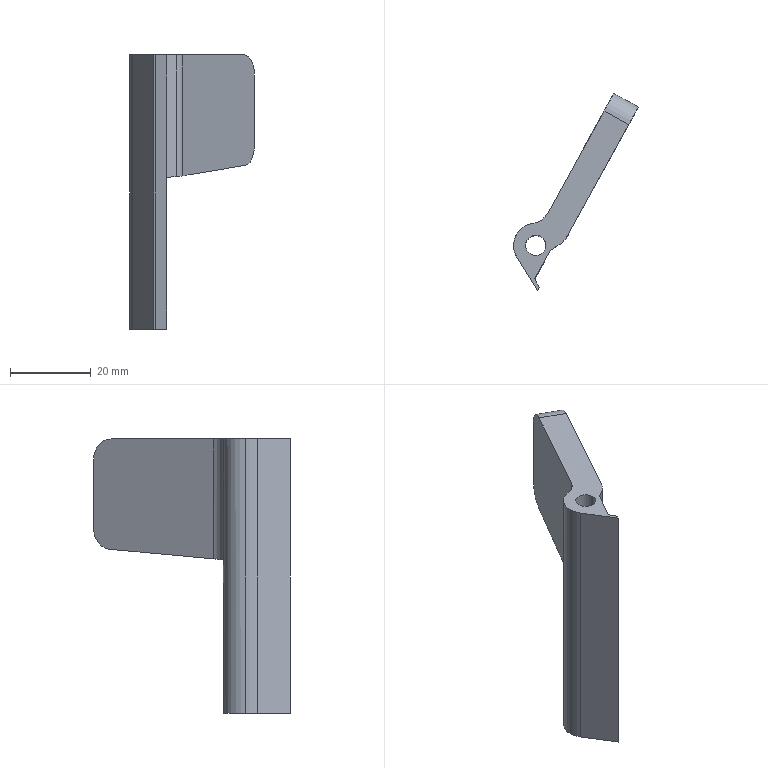Part | SolidWorks | features BaseBody 1 | 1 solid | 21 faces | box 30.974 x 48.805 x 68 mm | volume 12607 mm3 | plane 13 | cylinder 8 | commonest cylinder face diameters 10 x4 5 x2 11 x2
STEP:
#1=CARTESIAN_POINT('',(-2.751,-1.776,34.));
#2=VERTEX_POINT('',#1);
#3=CARTESIAN_POINT('',(-1.932,-4.664,34.));
#4=VERTEX_POINT('',#3);
#5=CARTESIAN_POINT('',(2.749,-1.776,34.));
#6=DIRECTION('',(0.,0.,1.));
#7=DIRECTION('',(-1.,0.,0.));
#8=AXIS2_PLACEMENT_3D('',#5,#6,#7);
#9=CIRCLE('',#8,5.5);
#10=EDGE_CURVE('',#2,#4,#9,.T.);
#11=ORIENTED_EDGE('',*,*,#10,.F.);
#12=CARTESIAN_POINT('',(-2.751,-1.776,-34.));
#13=VERTEX_POINT('',#12);
#14=CARTESIAN_POINT('',(-2.751,-1.776,34.));
#15=DIRECTION('',(0.,0.,-1.));
#16=VECTOR('',#15,1000.);
#17=LINE('',#14,#16);
#18=EDGE_CURVE('',#2,#13,#17,.T.);
#19=ORIENTED_EDGE('',*,*,#18,.T.);
#20=CARTESIAN_POINT('',(-1.932,-4.664,-34.));
#21=VERTEX_POINT('',#20);
#22=CARTESIAN_POINT('',(2.749,-1.776,-34.));
#23=DIRECTION('',(0.,0.,1.));
#24=DIRECTION('',(-1.,0.,0.));
#25=AXIS2_PLACEMENT_3D('',#22,#23,#24);
#26=CIRCLE('',#25,5.5);
#27=EDGE_CURVE('',#13,#21,#26,.T.);
#28=ORIENTED_EDGE('',*,*,#27,.T.);
#29=CARTESIAN_POINT('',(-1.932,-4.664,34.));
#30=DIRECTION('',(0.,0.,1.));
#31=VECTOR('',#30,1000.);
#32=LINE('',#29,#31);
#33=EDGE_CURVE('',#21,#4,#32,.T.);
#34=ORIENTED_EDGE('',*,*,#33,.T.);
#35=EDGE_LOOP('',(#11,#19,#28,#34));
#36=FACE_OUTER_BOUND('',#35,.T.);
#37=CARTESIAN_POINT('',(2.749,-1.776,34.));
#38=DIRECTION('',(0.,0.,-1.));
#39=DIRECTION('',(-1.,0.,0.));
#40=AXIS2_PLACEMENT_3D('',#37,#38,#39);
#41=CYLINDRICAL_SURFACE('',#40,5.5);
#42=ADVANCED_FACE('',(#36),#41,.T.);
#43=CARTESIAN_POINT('',(0.2488,-1.776,-34.));
#44=VERTEX_POINT('',#43);
#45=CARTESIAN_POINT('',(5.249,-1.776,-34.));
#46=VERTEX_POINT('',#45);
#47=CARTESIAN_POINT('',(2.749,-1.776,-34.));
#48=DIRECTION('',(0.,0.,1.));
#49=DIRECTION('',(1.,0.,0.));
#50=AXIS2_PLACEMENT_3D('',#47,#48,#49);
#51=CIRCLE('',#50,2.5);
#52=EDGE_CURVE('',#44,#46,#51,.T.);
#53=ORIENTED_EDGE('',*,*,#52,.F.);
#54=CARTESIAN_POINT('',(0.2488,-1.776,34.));
#55=VERTEX_POINT('',#54);
#56=CARTESIAN_POINT('',(0.2488,-1.776,-34.));
#57=DIRECTION('',(0.,0.,1.));
#58=VECTOR('',#57,1000.);
#59=LINE('',#56,#58);
#60=EDGE_CURVE('',#44,#55,#59,.T.);
#61=ORIENTED_EDGE('',*,*,#60,.T.);
#62=CARTESIAN_POINT('',(5.249,-1.776,34.));
#63=VERTEX_POINT('',#62);
#64=CARTESIAN_POINT('',(2.749,-1.776,34.));
#65=DIRECTION('',(0.,0.,-1.));
#66=DIRECTION('',(1.,0.,0.));
#67=AXIS2_PLACEMENT_3D('',#64,#65,#66);
#68=CIRCLE('',#67,2.5);
#69=EDGE_CURVE('',#63,#55,#68,.T.);
#70=ORIENTED_EDGE('',*,*,#69,.F.);
#71=CARTESIAN_POINT('',(5.249,-1.776,-34.));
#72=DIRECTION('',(0.,0.,1.));
#73=VECTOR('',#72,1000.);
#74=LINE('',#71,#73);
#75=EDGE_CURVE('',#46,#63,#74,.T.);
#76=ORIENTED_EDGE('',*,*,#75,.F.);
#77=EDGE_LOOP('',(#53,#61,#70,#76));
#78=FACE_OUTER_BOUND('',#77,.T.);
#79=CARTESIAN_POINT('',(2.749,-1.776,-34.));
#80=DIRECTION('',(0.,0.,1.));
#81=DIRECTION('',(1.,0.,0.));
#82=AXIS2_PLACEMENT_3D('',#79,#80,#81);
#83=CYLINDRICAL_SURFACE('',#82,2.5);
#84=ADVANCED_FACE('',(#78),#83,.F.);
#85=CARTESIAN_POINT('',(26.006,28.527,6.627));
#86=VERTEX_POINT('',#85);
#87=CARTESIAN_POINT('',(10.493,0.3506,4.019));
#88=VERTEX_POINT('',#87);
#89=CARTESIAN_POINT('',(26.006,28.527,6.627));
#90=DIRECTION('',(-0.4807,-0.8731,-0.08082));
#91=VECTOR('',#90,1000.);
#92=LINE('',#89,#91);
#93=EDGE_CURVE('',#86,#88,#92,.T.);
#94=ORIENTED_EDGE('',*,*,#93,.F.);
#95=CARTESIAN_POINT('',(28.223,32.553,11.611));
#96=VERTEX_POINT('',#95);
#97=CARTESIAN_POINT('',(25.811,28.173,11.611));
#98=DIRECTION('',(-0.876,0.4823,0.));
#99=DIRECTION('',(0.4823,0.876,0.));
#100=AXIS2_PLACEMENT_3D('',#97,#98,#99);
#101=CIRCLE('',#100,5.);
#102=EDGE_CURVE('',#96,#86,#101,.T.);
#103=ORIENTED_EDGE('',*,*,#102,.F.);
#104=CARTESIAN_POINT('',(28.223,32.553,29.));
#105=VERTEX_POINT('',#104);
#106=CARTESIAN_POINT('',(28.223,32.553,34.));
#107=DIRECTION('',(0.,0.,-1.));
#108=VECTOR('',#107,1000.);
#109=LINE('',#106,#108);
#110=EDGE_CURVE('',#105,#96,#109,.T.);
#111=ORIENTED_EDGE('',*,*,#110,.F.);
#112=CARTESIAN_POINT('',(25.811,28.173,34.));
#113=VERTEX_POINT('',#112);
#114=CARTESIAN_POINT('',(25.811,28.173,29.));
#115=DIRECTION('',(-0.876,0.4823,0.));
#116=DIRECTION('',(0.4823,0.876,0.));
#117=AXIS2_PLACEMENT_3D('',#114,#115,#116);
#118=CIRCLE('',#117,5.);
#119=EDGE_CURVE('',#113,#105,#118,.T.);
#120=ORIENTED_EDGE('',*,*,#119,.F.);
#121=CARTESIAN_POINT('',(10.493,0.3506,34.));
#122=VERTEX_POINT('',#121);
#123=CARTESIAN_POINT('',(28.223,32.553,34.));
#124=DIRECTION('',(0.4823,0.876,0.));
#125=VECTOR('',#124,1000.);
#126=LINE('',#123,#125);
#127=EDGE_CURVE('',#122,#113,#126,.T.);
#128=ORIENTED_EDGE('',*,*,#127,.F.);
#129=CARTESIAN_POINT('',(10.493,0.3506,34.));
#130=DIRECTION('',(0.,0.,1.));
#131=VECTOR('',#130,1000.);
#132=LINE('',#129,#131);
#133=EDGE_CURVE('',#88,#122,#132,.T.);
#134=ORIENTED_EDGE('',*,*,#133,.F.);
#135=EDGE_LOOP('',(#94,#103,#111,#120,#128,#134));
#136=FACE_OUTER_BOUND('',#135,.T.);
#137=CARTESIAN_POINT('',(28.223,32.553,34.));
#138=DIRECTION('',(-0.876,0.4823,0.));
#139=DIRECTION('',(-0.4823,-0.876,0.));
#140=AXIS2_PLACEMENT_3D('',#137,#138,#139);
#141=PLANE('',#140);
#142=ADVANCED_FACE('',(#136),#141,.F.);
#143=CARTESIAN_POINT('',(8.818,-1.443,34.));
#144=VERTEX_POINT('',#143);
#145=CARTESIAN_POINT('',(8.818,-1.443,3.827));
#146=VERTEX_POINT('',#145);
#147=CARTESIAN_POINT('',(8.818,-1.443,-47.577));
#148=DIRECTION('',(0.,0.,-1.));
#149=VECTOR('',#148,1000.);
#150=LINE('',#147,#149);
#151=EDGE_CURVE('',#144,#146,#150,.T.);
#152=ORIENTED_EDGE('',*,*,#151,.T.);
#153=CARTESIAN_POINT('',(8.818,-1.443,3.827));
#154=CARTESIAN_POINT('',(9.52,-0.9916,3.886));
#155=CARTESIAN_POINT('',(10.09,-0.3811,3.952));
#156=CARTESIAN_POINT('',(10.493,0.3506,4.019));
#157=(BOUNDED_CURVE()B_SPLINE_CURVE(3,(#153,#154,#155,#156),.UNSPECIFIED.,.F.,.F.)B_SPLINE_CURVE_WITH_KNOTS((4,4),(4.216,4.712),.UNSPECIFIED.)CURVE()GEOMETRIC_REPRESENTATION_ITEM()RATIONAL_B_SPLINE_CURVE((1.,0.9796,0.9796,1.))REPRESENTATION_ITEM(''));
#158=EDGE_CURVE('',#146,#88,#157,.T.);
#159=ORIENTED_EDGE('',*,*,#158,.T.);
#160=ORIENTED_EDGE('',*,*,#133,.T.);
#161=CARTESIAN_POINT('',(6.113,2.762,34.));
#162=DIRECTION('',(0.,0.,-1.));
#163=DIRECTION('',(1.,0.,0.));
#164=AXIS2_PLACEMENT_3D('',#161,#162,#163);
#165=CIRCLE('',#164,5.);
#166=EDGE_CURVE('',#122,#144,#165,.T.);
#167=ORIENTED_EDGE('',*,*,#166,.T.);
#168=EDGE_LOOP('',(#152,#159,#160,#167));
#169=FACE_OUTER_BOUND('',#168,.T.);
#170=CARTESIAN_POINT('',(6.113,2.762,-47.577));
#171=DIRECTION('',(0.,0.,1.));
#172=DIRECTION('',(1.,0.,0.));
#173=AXIS2_PLACEMENT_3D('',#170,#171,#172);
#174=CYLINDRICAL_SURFACE('',#173,5.);
#175=ADVANCED_FACE('',(#169),#174,.T.);
#176=CARTESIAN_POINT('',(4.245,3.517,4.));
#177=VERTEX_POINT('',#176);
#178=CARTESIAN_POINT('',(2.018,3.675,3.924));
#179=VERTEX_POINT('',#178);
#180=CARTESIAN_POINT('',(4.245,3.517,4.));
#181=CARTESIAN_POINT('',(3.519,3.722,3.986));
#182=CARTESIAN_POINT('',(2.766,3.776,3.961));
#183=CARTESIAN_POINT('',(2.018,3.675,3.924));
#184=(BOUNDED_CURVE()B_SPLINE_CURVE(3,(#180,#181,#182,#183),.UNSPECIFIED.,.F.,.F.)B_SPLINE_CURVE_WITH_KNOTS((4,4),(3.369,3.778),.UNSPECIFIED.)CURVE()GEOMETRIC_REPRESENTATION_ITEM()RATIONAL_B_SPLINE_CURVE((1.,0.9861,0.9861,1.))REPRESENTATION_ITEM(''));
#185=EDGE_CURVE('',#177,#179,#184,.T.);
#186=ORIENTED_EDGE('',*,*,#185,.T.);
#187=CARTESIAN_POINT('',(5.734,6.22,4.25));
#188=VERTEX_POINT('',#187);
#189=CARTESIAN_POINT('',(2.018,3.675,3.924));
#190=CARTESIAN_POINT('',(3.62,3.89,4.002));
#191=CARTESIAN_POINT('',(4.954,4.803,4.119));
#192=CARTESIAN_POINT('',(5.734,6.22,4.25));
#193=(BOUNDED_CURVE()B_SPLINE_CURVE(3,(#189,#190,#191,#192),.UNSPECIFIED.,.F.,.F.)B_SPLINE_CURVE_WITH_KNOTS((4,4),(0.6366,1.571),.UNSPECIFIED.)CURVE()GEOMETRIC_REPRESENTATION_ITEM()RATIONAL_B_SPLINE_CURVE((1.,0.9286,0.9286,1.))REPRESENTATION_ITEM(''));
#194=EDGE_CURVE('',#179,#188,#193,.T.);
#195=ORIENTED_EDGE('',*,*,#194,.T.);
#196=CARTESIAN_POINT('',(19.874,31.903,6.627));
#197=VERTEX_POINT('',#196);
#198=CARTESIAN_POINT('',(5.734,6.22,4.25));
#199=DIRECTION('',(0.4807,0.8731,0.08082));
#200=VECTOR('',#199,1000.);
#201=LINE('',#198,#200);
#202=EDGE_CURVE('',#188,#197,#201,.T.);
#203=ORIENTED_EDGE('',*,*,#202,.T.);
#204=CARTESIAN_POINT('',(19.874,31.903,6.627));
#205=DIRECTION('',(0.876,-0.4823,0.));
#206=VECTOR('',#205,1000.);
#207=LINE('',#204,#206);
#208=EDGE_CURVE('',#197,#86,#207,.T.);
#209=ORIENTED_EDGE('',*,*,#208,.T.);
#210=ORIENTED_EDGE('',*,*,#93,.T.);
#211=ORIENTED_EDGE('',*,*,#158,.F.);
#212=CARTESIAN_POINT('',(6.348,-3.031,3.617));
#213=VERTEX_POINT('',#212);
#214=CARTESIAN_POINT('',(8.818,-1.443,3.827));
#215=DIRECTION('',(-0.839,-0.5395,-0.07113));
#216=VECTOR('',#215,1000.);
#217=LINE('',#214,#216);
#218=EDGE_CURVE('',#146,#213,#217,.T.);
#219=ORIENTED_EDGE('',*,*,#218,.T.);
#220=CARTESIAN_POINT('',(6.421,2.319,4.));
#221=VERTEX_POINT('',#220);
#222=CARTESIAN_POINT('',(6.348,-3.031,3.617));
#223=DIRECTION('',(0.01357,0.9974,0.07137));
#224=VECTOR('',#223,1000.);
#225=LINE('',#222,#224);
#226=EDGE_CURVE('',#213,#221,#225,.T.);
#227=ORIENTED_EDGE('',*,*,#226,.T.);
#228=CARTESIAN_POINT('',(6.421,2.319,4.));
#229=DIRECTION('',(-0.876,0.4823,0.));
#230=VECTOR('',#229,1000.);
#231=LINE('',#228,#230);
#232=EDGE_CURVE('',#221,#177,#231,.T.);
#233=ORIENTED_EDGE('',*,*,#232,.T.);
#234=EDGE_LOOP('',(#186,#195,#203,#209,#210,#211,#219,#227,#233));
#235=FACE_OUTER_BOUND('',#234,.T.);
#236=CARTESIAN_POINT('',(21.765,-6.13,4.));
#237=DIRECTION('',(0.03898,0.07079,-0.9967));
#238=DIRECTION('',(0.,0.9975,0.07085));
#239=AXIS2_PLACEMENT_3D('',#236,#237,#238);
#240=PLANE('',#239);
#241=ADVANCED_FACE('',(#235),#240,.T.);
#242=ORIENTED_EDGE('',*,*,#102,.T.);
#243=ORIENTED_EDGE('',*,*,#208,.F.);
#244=CARTESIAN_POINT('',(22.091,35.929,11.611));
#245=VERTEX_POINT('',#244);
#246=CARTESIAN_POINT('',(19.679,31.549,11.611));
#247=DIRECTION('',(0.876,-0.4823,0.));
#248=DIRECTION('',(0.4823,0.876,0.));
#249=AXIS2_PLACEMENT_3D('',#246,#247,#248);
#250=CIRCLE('',#249,5.);
#251=EDGE_CURVE('',#197,#245,#250,.T.);
#252=ORIENTED_EDGE('',*,*,#251,.T.);
#253=CARTESIAN_POINT('',(28.223,32.553,11.611));
#254=DIRECTION('',(0.876,-0.4823,0.));
#255=VECTOR('',#254,1000.);
#256=LINE('',#253,#255);
#257=EDGE_CURVE('',#245,#96,#256,.T.);
#258=ORIENTED_EDGE('',*,*,#257,.T.);
#259=EDGE_LOOP('',(#242,#243,#252,#258));
#260=FACE_OUTER_BOUND('',#259,.T.);
#261=CARTESIAN_POINT('',(25.811,28.173,11.611));
#262=DIRECTION('',(0.876,-0.4823,0.));
#263=DIRECTION('',(0.4823,0.876,0.));
#264=AXIS2_PLACEMENT_3D('',#261,#262,#263);
#265=CYLINDRICAL_SURFACE('',#264,5.);
#266=ADVANCED_FACE('',(#260),#265,.T.);
#267=CARTESIAN_POINT('',(22.091,35.929,29.));
#268=VERTEX_POINT('',#267);
#269=CARTESIAN_POINT('',(22.091,35.929,34.));
#270=DIRECTION('',(0.,0.,-1.));
#271=VECTOR('',#270,1000.);
#272=LINE('',#269,#271);
#273=EDGE_CURVE('',#268,#245,#272,.T.);
#274=ORIENTED_EDGE('',*,*,#273,.F.);
#275=CARTESIAN_POINT('',(28.223,32.553,29.));
#276=DIRECTION('',(-0.876,0.4823,0.));
#277=VECTOR('',#276,1000.);
#278=LINE('',#275,#277);
#279=EDGE_CURVE('',#105,#268,#278,.T.);
#280=ORIENTED_EDGE('',*,*,#279,.F.);
#281=ORIENTED_EDGE('',*,*,#110,.T.);
#282=ORIENTED_EDGE('',*,*,#257,.F.);
#283=EDGE_LOOP('',(#274,#280,#281,#282));
#284=FACE_OUTER_BOUND('',#283,.T.);
#285=CARTESIAN_POINT('',(28.223,32.553,34.));
#286=DIRECTION('',(-0.4823,-0.876,0.));
#287=DIRECTION('',(0.876,-0.4823,0.));
#288=AXIS2_PLACEMENT_3D('',#285,#286,#287);
#289=PLANE('',#288);
#290=ADVANCED_FACE('',(#284),#289,.F.);
#291=ORIENTED_EDGE('',*,*,#119,.T.);
#292=ORIENTED_EDGE('',*,*,#279,.T.);
#293=CARTESIAN_POINT('',(19.679,31.549,34.));
#294=VERTEX_POINT('',#293);
#295=CARTESIAN_POINT('',(19.679,31.549,29.));
#296=DIRECTION('',(0.876,-0.4823,0.));
#297=DIRECTION('',(0.4823,0.876,0.));
#298=AXIS2_PLACEMENT_3D('',#295,#296,#297);
#299=CIRCLE('',#298,5.);
#300=EDGE_CURVE('',#268,#294,#299,.T.);
#301=ORIENTED_EDGE('',*,*,#300,.T.);
#302=CARTESIAN_POINT('',(20.767,30.95,34.));
#303=DIRECTION('',(0.876,-0.4823,0.));
#304=VECTOR('',#303,1000.);
#305=LINE('',#302,#304);
#306=EDGE_CURVE('',#294,#113,#305,.T.);
#307=ORIENTED_EDGE('',*,*,#306,.T.);
#308=EDGE_LOOP('',(#291,#292,#301,#307));
#309=FACE_OUTER_BOUND('',#308,.T.);
#310=CARTESIAN_POINT('',(20.767,30.95,29.));
#311=DIRECTION('',(0.876,-0.4823,0.));
#312=DIRECTION('',(0.4823,0.876,0.));
#313=AXIS2_PLACEMENT_3D('',#310,#311,#312);
#314=CYLINDRICAL_SURFACE('',#313,5.);
#315=ADVANCED_FACE('',(#309),#314,.T.);
#316=CARTESIAN_POINT('',(3.211,-12.876,34.));
#317=VERTEX_POINT('',#316);
#318=CARTESIAN_POINT('',(-1.932,-4.664,34.));
#319=DIRECTION('',(0.5308,-0.8475,0.));
#320=VECTOR('',#319,1000.);
#321=LINE('',#318,#320);
#322=EDGE_CURVE('',#4,#317,#321,.T.);
#323=ORIENTED_EDGE('',*,*,#322,.T.);
#324=CARTESIAN_POINT('',(3.612,-12.147,34.));
#325=VERTEX_POINT('',#324);
#326=CARTESIAN_POINT('',(28.223,32.553,34.));
#327=DIRECTION('',(0.4823,0.876,0.));
#328=VECTOR('',#327,1000.);
#329=LINE('',#326,#328);
#330=EDGE_CURVE('',#317,#325,#329,.T.);
#331=ORIENTED_EDGE('',*,*,#330,.T.);
#332=CARTESIAN_POINT('',(2.489,-10.039,34.));
#333=VERTEX_POINT('',#332);
#334=CARTESIAN_POINT('',(3.612,-12.147,34.));
#335=DIRECTION('',(-0.4703,0.8825,0.));
#336=VECTOR('',#335,1000.);
#337=LINE('',#334,#336);
#338=EDGE_CURVE('',#325,#333,#337,.T.);
#339=ORIENTED_EDGE('',*,*,#338,.T.);
#340=CARTESIAN_POINT('',(6.348,-3.031,34.));
#341=VERTEX_POINT('',#340);
#342=CARTESIAN_POINT('',(2.489,-10.039,34.));
#343=DIRECTION('',(0.4823,0.876,0.));
#344=VECTOR('',#343,1000.);
#345=LINE('',#342,#344);
#346=EDGE_CURVE('',#333,#341,#345,.T.);
#347=ORIENTED_EDGE('',*,*,#346,.T.);
#348=CARTESIAN_POINT('',(6.348,-3.031,34.));
#349=DIRECTION('',(0.8411,0.5409,0.));
#350=VECTOR('',#349,1000.);
#351=LINE('',#348,#350);
#352=EDGE_CURVE('',#341,#144,#351,.T.);
#353=ORIENTED_EDGE('',*,*,#352,.T.);
#354=ORIENTED_EDGE('',*,*,#166,.F.);
#355=ORIENTED_EDGE('',*,*,#127,.T.);
#356=ORIENTED_EDGE('',*,*,#306,.F.);
#357=CARTESIAN_POINT('',(5.734,6.22,34.));
#358=VERTEX_POINT('',#357);
#359=CARTESIAN_POINT('',(19.679,31.549,34.));
#360=DIRECTION('',(-0.4823,-0.876,0.));
#361=VECTOR('',#360,1000.);
#362=LINE('',#359,#361);
#363=EDGE_CURVE('',#294,#358,#362,.T.);
#364=ORIENTED_EDGE('',*,*,#363,.T.);
#365=CARTESIAN_POINT('',(2.018,3.675,34.));
#366=VERTEX_POINT('',#365);
#367=CARTESIAN_POINT('',(1.354,8.631,34.));
#368=DIRECTION('',(0.,0.,-1.));
#369=DIRECTION('',(-1.,0.,0.));
#370=AXIS2_PLACEMENT_3D('',#367,#368,#369);
#371=CIRCLE('',#370,5.);
#372=EDGE_CURVE('',#358,#366,#371,.T.);
#373=ORIENTED_EDGE('',*,*,#372,.T.);
#374=CARTESIAN_POINT('',(2.749,-1.776,34.));
#375=DIRECTION('',(0.,0.,1.));
#376=DIRECTION('',(-1.,0.,0.));
#377=AXIS2_PLACEMENT_3D('',#374,#375,#376);
#378=CIRCLE('',#377,5.5);
#379=EDGE_CURVE('',#366,#2,#378,.T.);
#380=ORIENTED_EDGE('',*,*,#379,.T.);
#381=ORIENTED_EDGE('',*,*,#10,.T.);
#382=EDGE_LOOP('',(#323,#331,#339,#347,#353,#354,#355,#356,#364,#373,#380,#381));
#383=FACE_OUTER_BOUND('',#382,.T.);
#384=ORIENTED_EDGE('',*,*,#69,.T.);
#385=CARTESIAN_POINT('',(2.749,-1.776,34.));
#386=DIRECTION('',(0.,0.,-1.));
#387=DIRECTION('',(1.,0.,0.));
#388=AXIS2_PLACEMENT_3D('',#385,#386,#387);
#389=CIRCLE('',#388,2.5);
#390=EDGE_CURVE('',#55,#63,#389,.T.);
#391=ORIENTED_EDGE('',*,*,#390,.T.);
#392=EDGE_LOOP('',(#384,#391));
#393=FACE_BOUND('',#392,.T.);
#394=CARTESIAN_POINT('',(2.749,-1.776,34.));
#395=DIRECTION('',(0.,0.,1.));
#396=DIRECTION('',(1.,0.,0.));
#397=AXIS2_PLACEMENT_3D('',#394,#395,#396);
#398=PLANE('',#397);
#399=ADVANCED_FACE('',(#383,#393),#398,.T.);
#400=ORIENTED_EDGE('',*,*,#352,.F.);
#401=CARTESIAN_POINT('',(6.348,-3.031,-47.577));
#402=DIRECTION('',(0.,0.,1.));
#403=VECTOR('',#402,1000.);
#404=LINE('',#401,#403);
#405=EDGE_CURVE('',#213,#341,#404,.T.);
#406=ORIENTED_EDGE('',*,*,#405,.F.);
#407=ORIENTED_EDGE('',*,*,#218,.F.);
#408=ORIENTED_EDGE('',*,*,#151,.F.);
#409=EDGE_LOOP('',(#400,#406,#407,#408));
#410=FACE_OUTER_BOUND('',#409,.T.);
#411=CARTESIAN_POINT('',(6.348,-3.031,-47.577));
#412=DIRECTION('',(-0.5409,0.8411,0.));
#413=DIRECTION('',(-0.8411,-0.5409,0.));
#414=AXIS2_PLACEMENT_3D('',#411,#412,#413);
#415=PLANE('',#414);
#416=ADVANCED_FACE('',(#410),#415,.F.);
#417=ORIENTED_EDGE('',*,*,#194,.F.);
#418=CARTESIAN_POINT('',(2.018,3.675,34.));
#419=DIRECTION('',(0.,0.,-1.));
#420=VECTOR('',#419,1000.);
#421=LINE('',#418,#420);
#422=EDGE_CURVE('',#366,#179,#421,.T.);
#423=ORIENTED_EDGE('',*,*,#422,.F.);
#424=ORIENTED_EDGE('',*,*,#372,.F.);
#425=CARTESIAN_POINT('',(5.734,6.22,34.));
#426=DIRECTION('',(0.,0.,1.));
#427=VECTOR('',#426,1000.);
#428=LINE('',#425,#427);
#429=EDGE_CURVE('',#188,#358,#428,.T.);
#430=ORIENTED_EDGE('',*,*,#429,.F.);
#431=EDGE_LOOP('',(#417,#423,#424,#430));
#432=FACE_OUTER_BOUND('',#431,.T.);
#433=CARTESIAN_POINT('',(1.354,8.631,34.));
#434=DIRECTION('',(0.,0.,-1.));
#435=DIRECTION('',(-1.,0.,0.));
#436=AXIS2_PLACEMENT_3D('',#433,#434,#435);
#437=CYLINDRICAL_SURFACE('',#436,5.);
#438=ADVANCED_FACE('',(#432),#437,.F.);
#439=ORIENTED_EDGE('',*,*,#18,.F.);
#440=ORIENTED_EDGE('',*,*,#379,.F.);
#441=ORIENTED_EDGE('',*,*,#422,.T.);
#442=ORIENTED_EDGE('',*,*,#185,.F.);
#443=CARTESIAN_POINT('',(4.245,3.517,-34.));
#444=VERTEX_POINT('',#443);
#445=CARTESIAN_POINT('',(4.245,3.517,34.));
#446=DIRECTION('',(0.,0.,-1.));
#447=VECTOR('',#446,1000.);
#448=LINE('',#445,#447);
#449=EDGE_CURVE('',#177,#444,#448,.T.);
#450=ORIENTED_EDGE('',*,*,#449,.T.);
#451=CARTESIAN_POINT('',(2.749,-1.776,-34.));
#452=DIRECTION('',(0.,0.,1.));
#453=DIRECTION('',(-1.,0.,0.));
#454=AXIS2_PLACEMENT_3D('',#451,#452,#453);
#455=CIRCLE('',#454,5.5);
#456=EDGE_CURVE('',#444,#13,#455,.T.);
#457=ORIENTED_EDGE('',*,*,#456,.T.);
#458=EDGE_LOOP('',(#439,#440,#441,#442,#450,#457));
#459=FACE_OUTER_BOUND('',#458,.T.);
#460=CARTESIAN_POINT('',(2.749,-1.776,34.));
#461=DIRECTION('',(0.,0.,-1.));
#462=DIRECTION('',(-1.,0.,0.));
#463=AXIS2_PLACEMENT_3D('',#460,#461,#462);
#464=CYLINDRICAL_SURFACE('',#463,5.5);
#465=ADVANCED_FACE('',(#459),#464,.T.);
#466=CARTESIAN_POINT('',(6.421,2.319,-34.));
#467=VERTEX_POINT('',#466);
#468=CARTESIAN_POINT('',(6.421,2.319,4.));
#469=DIRECTION('',(0.,0.,-1.));
#470=VECTOR('',#469,1000.);
#471=LINE('',#468,#470);
#472=EDGE_CURVE('',#221,#467,#471,.T.);
#473=ORIENTED_EDGE('',*,*,#472,.T.);
#474=CARTESIAN_POINT('',(21.765,-6.13,-34.));
#475=DIRECTION('',(-0.876,0.4823,0.));
#476=VECTOR('',#475,1000.);
#477=LINE('',#474,#476);
#478=EDGE_CURVE('',#467,#444,#477,.T.);
#479=ORIENTED_EDGE('',*,*,#478,.T.);
#480=ORIENTED_EDGE('',*,*,#449,.F.);
#481=ORIENTED_EDGE('',*,*,#232,.F.);
#482=EDGE_LOOP('',(#473,#479,#480,#481));
#483=FACE_OUTER_BOUND('',#482,.T.);
#484=CARTESIAN_POINT('',(21.765,-6.13,4.));
#485=DIRECTION('',(0.4823,0.876,0.));
#486=DIRECTION('',(-0.876,0.4823,0.));
#487=AXIS2_PLACEMENT_3D('',#484,#485,#486);
#488=PLANE('',#487);
#489=ADVANCED_FACE('',(#483),#488,.T.);
#490=CARTESIAN_POINT('',(6.348,-3.031,-34.));
#491=VERTEX_POINT('',#490);
#492=CARTESIAN_POINT('',(6.348,-3.031,-34.));
#493=DIRECTION('',(-0.01361,-0.9999,0.));
#494=VECTOR('',#493,1000.);
#495=LINE('',#492,#494);
#496=EDGE_CURVE('',#467,#491,#495,.T.);
#497=ORIENTED_EDGE('',*,*,#496,.F.);
#498=ORIENTED_EDGE('',*,*,#472,.F.);
#499=ORIENTED_EDGE('',*,*,#226,.F.);
#500=CARTESIAN_POINT('',(6.348,-3.031,11.818));
#501=DIRECTION('',(0.,0.,1.));
#502=VECTOR('',#501,1000.);
#503=LINE('',#500,#502);
#504=EDGE_CURVE('',#491,#213,#503,.T.);
#505=ORIENTED_EDGE('',*,*,#504,.F.);
#506=EDGE_LOOP('',(#497,#498,#499,#505));
#507=FACE_OUTER_BOUND('',#506,.T.);
#508=CARTESIAN_POINT('',(6.348,-3.031,11.818));
#509=DIRECTION('',(-0.9999,0.01361,0.));
#510=DIRECTION('',(-0.01361,-0.9999,0.));
#511=AXIS2_PLACEMENT_3D('',#508,#509,#510);
#512=PLANE('',#511);
#513=ADVANCED_FACE('',(#507),#512,.F.);
#514=ORIENTED_EDGE('',*,*,#202,.F.);
#515=ORIENTED_EDGE('',*,*,#429,.T.);
#516=ORIENTED_EDGE('',*,*,#363,.F.);
#517=ORIENTED_EDGE('',*,*,#300,.F.);
#518=ORIENTED_EDGE('',*,*,#273,.T.);
#519=ORIENTED_EDGE('',*,*,#251,.F.);
#520=EDGE_LOOP('',(#514,#515,#516,#517,#518,#519));
#521=FACE_OUTER_BOUND('',#520,.T.);
#522=CARTESIAN_POINT('',(4.245,3.517,34.));
#523=DIRECTION('',(0.876,-0.4823,0.));
#524=DIRECTION('',(0.4823,0.876,0.));
#525=AXIS2_PLACEMENT_3D('',#522,#523,#524);
#526=PLANE('',#525);
#527=ADVANCED_FACE('',(#521),#526,.F.);
#528=ORIENTED_EDGE('',*,*,#322,.F.);
#529=ORIENTED_EDGE('',*,*,#33,.F.);
#530=CARTESIAN_POINT('',(3.211,-12.876,-34.));
#531=VERTEX_POINT('',#530);
#532=CARTESIAN_POINT('',(-1.932,-4.664,-34.));
#533=DIRECTION('',(-0.5308,0.8475,0.));
#534=VECTOR('',#533,1000.);
#535=LINE('',#532,#534);
#536=EDGE_CURVE('',#531,#21,#535,.T.);
#537=ORIENTED_EDGE('',*,*,#536,.F.);
#538=CARTESIAN_POINT('',(3.211,-12.876,34.));
#539=DIRECTION('',(0.,0.,-1.));
#540=VECTOR('',#539,1000.);
#541=LINE('',#538,#540);
#542=EDGE_CURVE('',#317,#531,#541,.T.);
#543=ORIENTED_EDGE('',*,*,#542,.F.);
#544=EDGE_LOOP('',(#528,#529,#537,#543));
#545=FACE_OUTER_BOUND('',#544,.T.);
#546=CARTESIAN_POINT('',(-1.932,-4.664,34.));
#547=DIRECTION('',(0.8475,0.5308,0.));
#548=DIRECTION('',(-0.5308,0.8475,0.));
#549=AXIS2_PLACEMENT_3D('',#546,#547,#548);
#550=PLANE('',#549);
#551=ADVANCED_FACE('',(#545),#550,.F.);
#552=ORIENTED_EDGE('',*,*,#405,.T.);
#553=ORIENTED_EDGE('',*,*,#346,.F.);
#554=CARTESIAN_POINT('',(2.489,-10.039,-34.));
#555=VERTEX_POINT('',#554);
#556=CARTESIAN_POINT('',(2.489,-10.039,-47.577));
#557=DIRECTION('',(0.,0.,1.));
#558=VECTOR('',#557,1000.);
#559=LINE('',#556,#558);
#560=EDGE_CURVE('',#555,#333,#559,.T.);
#561=ORIENTED_EDGE('',*,*,#560,.F.);
#562=CARTESIAN_POINT('',(2.489,-10.039,-34.));
#563=DIRECTION('',(-0.4823,-0.876,0.));
#564=VECTOR('',#563,1000.);
#565=LINE('',#562,#564);
#566=EDGE_CURVE('',#491,#555,#565,.T.);
#567=ORIENTED_EDGE('',*,*,#566,.F.);
#568=ORIENTED_EDGE('',*,*,#504,.T.);
#569=EDGE_LOOP('',(#552,#553,#561,#567,#568));
#570=FACE_OUTER_BOUND('',#569,.T.);
#571=CARTESIAN_POINT('',(2.489,-10.039,-47.577));
#572=DIRECTION('',(-0.876,0.4823,0.));
#573=DIRECTION('',(-0.4823,-0.876,0.));
#574=AXIS2_PLACEMENT_3D('',#571,#572,#573);
#575=PLANE('',#574);
#576=ADVANCED_FACE('',(#570),#575,.F.);
#577=ORIENTED_EDGE('',*,*,#338,.F.);
#578=CARTESIAN_POINT('',(3.612,-12.147,-34.));
#579=VERTEX_POINT('',#578);
#580=CARTESIAN_POINT('',(3.612,-12.147,-47.577));
#581=DIRECTION('',(0.,0.,1.));
#582=VECTOR('',#581,1000.);
#583=LINE('',#580,#582);
#584=EDGE_CURVE('',#579,#325,#583,.T.);
#585=ORIENTED_EDGE('',*,*,#584,.F.);
#586=CARTESIAN_POINT('',(3.612,-12.147,-34.));
#587=DIRECTION('',(0.4703,-0.8825,0.));
#588=VECTOR('',#587,1000.);
#589=LINE('',#586,#588);
#590=EDGE_CURVE('',#555,#579,#589,.T.);
#591=ORIENTED_EDGE('',*,*,#590,.F.);
#592=ORIENTED_EDGE('',*,*,#560,.T.);
#593=EDGE_LOOP('',(#577,#585,#591,#592));
#594=FACE_OUTER_BOUND('',#593,.T.);
#595=CARTESIAN_POINT('',(3.612,-12.147,-47.577));
#596=DIRECTION('',(-0.8825,-0.4703,0.));
#597=DIRECTION('',(0.4703,-0.8825,0.));
#598=AXIS2_PLACEMENT_3D('',#595,#596,#597);
#599=PLANE('',#598);
#600=ADVANCED_FACE('',(#594),#599,.F.);
#601=ORIENTED_EDGE('',*,*,#60,.F.);
#602=CARTESIAN_POINT('',(2.749,-1.776,-34.));
#603=DIRECTION('',(0.,0.,1.));
#604=DIRECTION('',(1.,0.,0.));
#605=AXIS2_PLACEMENT_3D('',#602,#603,#604);
#606=CIRCLE('',#605,2.5);
#607=EDGE_CURVE('',#46,#44,#606,.T.);
#608=ORIENTED_EDGE('',*,*,#607,.F.);
#609=ORIENTED_EDGE('',*,*,#75,.T.);
#610=ORIENTED_EDGE('',*,*,#390,.F.);
#611=EDGE_LOOP('',(#601,#608,#609,#610));
#612=FACE_OUTER_BOUND('',#611,.T.);
#613=CARTESIAN_POINT('',(2.749,-1.776,-34.));
#614=DIRECTION('',(0.,0.,1.));
#615=DIRECTION('',(1.,0.,0.));
#616=AXIS2_PLACEMENT_3D('',#613,#614,#615);
#617=CYLINDRICAL_SURFACE('',#616,2.5);
#618=ADVANCED_FACE('',(#612),#617,.F.);
#619=ORIENTED_EDGE('',*,*,#607,.T.);
#620=ORIENTED_EDGE('',*,*,#52,.T.);
#621=EDGE_LOOP('',(#619,#620));
#622=FACE_BOUND('',#621,.T.);
#623=ORIENTED_EDGE('',*,*,#566,.T.);
#624=ORIENTED_EDGE('',*,*,#590,.T.);
#625=CARTESIAN_POINT('',(3.211,-12.876,-34.));
#626=DIRECTION('',(0.4823,0.876,0.));
#627=VECTOR('',#626,1000.);
#628=LINE('',#625,#627);
#629=EDGE_CURVE('',#531,#579,#628,.T.);
#630=ORIENTED_EDGE('',*,*,#629,.F.);
#631=ORIENTED_EDGE('',*,*,#536,.T.);
#632=ORIENTED_EDGE('',*,*,#27,.F.);
#633=ORIENTED_EDGE('',*,*,#456,.F.);
#634=ORIENTED_EDGE('',*,*,#478,.F.);
#635=ORIENTED_EDGE('',*,*,#496,.T.);
#636=EDGE_LOOP('',(#623,#624,#630,#631,#632,#633,#634,#635));
#637=FACE_OUTER_BOUND('',#636,.T.);
#638=CARTESIAN_POINT('',(2.749,-1.776,-34.));
#639=DIRECTION('',(0.,0.,1.));
#640=DIRECTION('',(1.,0.,0.));
#641=AXIS2_PLACEMENT_3D('',#638,#639,#640);
#642=PLANE('',#641);
#643=ADVANCED_FACE('',(#622,#637),#642,.F.);
#644=ORIENTED_EDGE('',*,*,#330,.F.);
#645=ORIENTED_EDGE('',*,*,#542,.T.);
#646=ORIENTED_EDGE('',*,*,#629,.T.);
#647=ORIENTED_EDGE('',*,*,#584,.T.);
#648=EDGE_LOOP('',(#644,#645,#646,#647));
#649=FACE_OUTER_BOUND('',#648,.T.);
#650=CARTESIAN_POINT('',(28.223,32.553,34.));
#651=DIRECTION('',(-0.876,0.4823,0.));
#652=DIRECTION('',(-0.4823,-0.876,0.));
#653=AXIS2_PLACEMENT_3D('',#650,#651,#652);
#654=PLANE('',#653);
#655=ADVANCED_FACE('',(#649),#654,.F.);
#656=CLOSED_SHELL('',(#42,#84,#142,#175,#241,#266,#290,#315,#399,#416,#438,#465,#489,#513,#527,#551,#576,#600,#618,#643,#655));
#657=MANIFOLD_SOLID_BREP('',#656);
#658=CARTESIAN_POINT('',(0.,0.,0.));
#659=DIRECTION('',(0.,0.,1.));
#660=DIRECTION('',(1.,0.,0.));
#661=AXIS2_PLACEMENT_3D('',#658,#659,#660);
#662=(LENGTH_UNIT()NAMED_UNIT(*)SI_UNIT(.MILLI.,.METRE.));
#663=UNCERTAINTY_MEASURE_WITH_UNIT(LENGTH_MEASURE(0.00001),#662,'','');
#664=(NAMED_UNIT(*)PLANE_ANGLE_UNIT()SI_UNIT($,.RADIAN.));
#665=(NAMED_UNIT(*)SI_UNIT($,.STERADIAN.)SOLID_ANGLE_UNIT());
#666=(GEOMETRIC_REPRESENTATION_CONTEXT(3)GLOBAL_UNCERTAINTY_ASSIGNED_CONTEXT((#663))GLOBAL_UNIT_ASSIGNED_CONTEXT((#662,#664,#665))REPRESENTATION_CONTEXT('',''));
#667=ADVANCED_BREP_SHAPE_REPRESENTATION('',(#657,#661),#666);